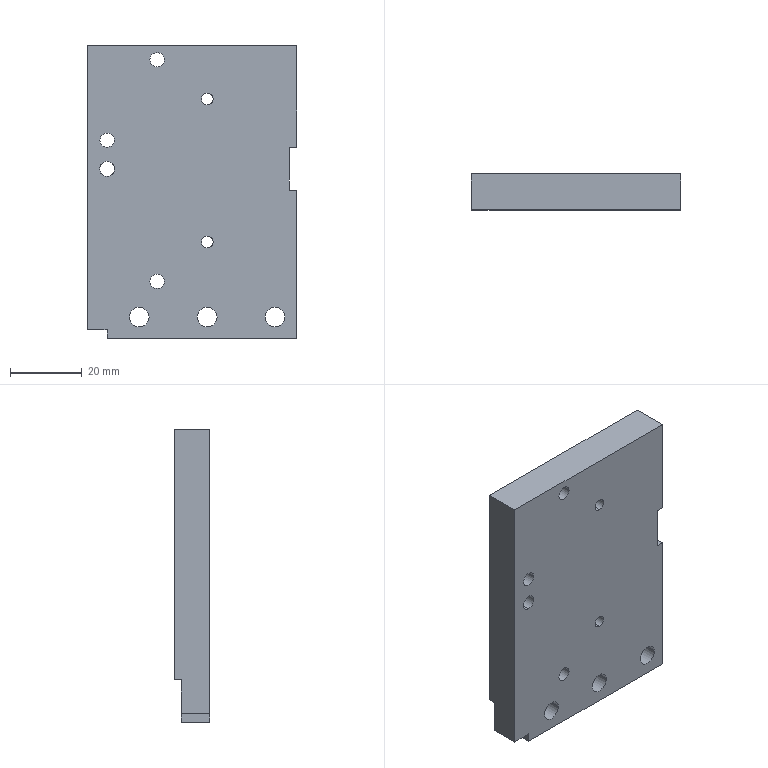Part | NX | 1 solid | 56 faces | box 58.5 x 10 x 82 mm | volume 44523 mm3 | cylinder 24 | cone 18 | plane 14 | commonest cylinder face diameters 3.3 x8 4 x6 5.5 x6 4.2 x4